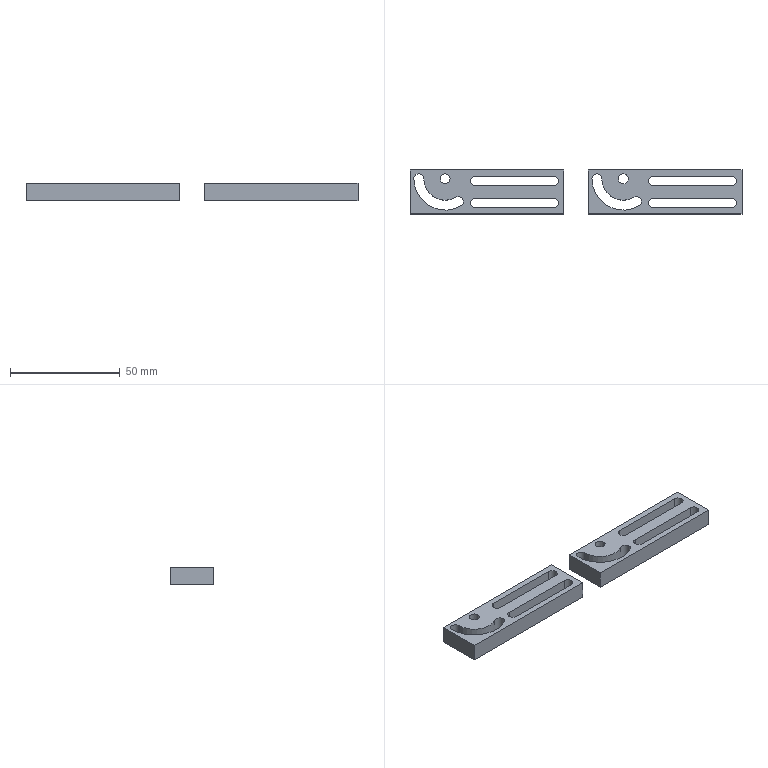Part | NX | 2 solids | 38 faces | box 151 x 20 x 8 mm | volume 14461 mm3 | plane 20 | cylinder 18 | commonest cylinder face diameters 4.5 x14 19.5 x2 28.5 x2
STEP:
#1=CARTESIAN_POINT('',(23.125,3.659,0.));
#2=VERTEX_POINT('',#1);
#3=CARTESIAN_POINT('',(1.75,16.,0.));
#4=VERTEX_POINT('',#3);
#5=CARTESIAN_POINT('',(16.,16.,0.));
#6=DIRECTION('',(0.,0.,-1.));
#7=DIRECTION('',(-1.,0.,0.));
#8=AXIS2_PLACEMENT_3D('',#5,#6,#7);
#9=CIRCLE('',#8,14.25);
#10=EDGE_CURVE('',#2,#4,#9,.T.);
#11=ORIENTED_EDGE('',*,*,#10,.T.);
#12=CARTESIAN_POINT('',(1.75,16.,8.));
#13=VERTEX_POINT('',#12);
#14=CARTESIAN_POINT('',(1.75,16.,8.));
#15=DIRECTION('',(0.,0.,-1.));
#16=VECTOR('',#15,1000.);
#17=LINE('',#14,#16);
#18=EDGE_CURVE('',#13,#4,#17,.T.);
#19=ORIENTED_EDGE('',*,*,#18,.F.);
#20=CARTESIAN_POINT('',(23.125,3.659,8.));
#21=VERTEX_POINT('',#20);
#22=CARTESIAN_POINT('',(16.,16.,8.));
#23=DIRECTION('',(0.,0.,-1.));
#24=DIRECTION('',(-1.,0.,0.));
#25=AXIS2_PLACEMENT_3D('',#22,#23,#24);
#26=CIRCLE('',#25,14.25);
#27=EDGE_CURVE('',#21,#13,#26,.T.);
#28=ORIENTED_EDGE('',*,*,#27,.F.);
#29=CARTESIAN_POINT('',(23.125,3.659,8.));
#30=DIRECTION('',(0.,0.,-1.));
#31=VECTOR('',#30,1000.);
#32=LINE('',#29,#31);
#33=EDGE_CURVE('',#21,#2,#32,.T.);
#34=ORIENTED_EDGE('',*,*,#33,.T.);
#35=EDGE_LOOP('',(#11,#19,#28,#34));
#36=FACE_BOUND('',#35,.T.);
#37=CARTESIAN_POINT('',(16.,16.,8.));
#38=DIRECTION('',(0.,0.,-1.));
#39=DIRECTION('',(-1.,0.,0.));
#40=AXIS2_PLACEMENT_3D('',#37,#38,#39);
#41=CYLINDRICAL_SURFACE('',#40,14.25);
#42=ADVANCED_FACE('',(#36),#41,.F.);
#43=CARTESIAN_POINT('',(6.25,16.,0.));
#44=VERTEX_POINT('',#43);
#45=CARTESIAN_POINT('',(4.,16.,0.));
#46=DIRECTION('',(0.,0.,-1.));
#47=DIRECTION('',(-1.,0.,0.));
#48=AXIS2_PLACEMENT_3D('',#45,#46,#47);
#49=CIRCLE('',#48,2.25);
#50=EDGE_CURVE('',#4,#44,#49,.T.);
#51=ORIENTED_EDGE('',*,*,#50,.T.);
#52=CARTESIAN_POINT('',(6.25,16.,8.));
#53=VERTEX_POINT('',#52);
#54=CARTESIAN_POINT('',(6.25,16.,8.));
#55=DIRECTION('',(0.,0.,-1.));
#56=VECTOR('',#55,1000.);
#57=LINE('',#54,#56);
#58=EDGE_CURVE('',#53,#44,#57,.T.);
#59=ORIENTED_EDGE('',*,*,#58,.F.);
#60=CARTESIAN_POINT('',(4.,16.,8.));
#61=DIRECTION('',(0.,0.,-1.));
#62=DIRECTION('',(-1.,0.,0.));
#63=AXIS2_PLACEMENT_3D('',#60,#61,#62);
#64=CIRCLE('',#63,2.25);
#65=EDGE_CURVE('',#13,#53,#64,.T.);
#66=ORIENTED_EDGE('',*,*,#65,.F.);
#67=ORIENTED_EDGE('',*,*,#18,.T.);
#68=EDGE_LOOP('',(#51,#59,#66,#67));
#69=FACE_BOUND('',#68,.T.);
#70=CARTESIAN_POINT('',(4.,16.,8.));
#71=DIRECTION('',(0.,0.,-1.));
#72=DIRECTION('',(-1.,0.,0.));
#73=AXIS2_PLACEMENT_3D('',#70,#71,#72);
#74=CYLINDRICAL_SURFACE('',#73,2.25);
#75=ADVANCED_FACE('',(#69),#74,.F.);
#76=CARTESIAN_POINT('',(20.875,7.556,0.));
#77=VERTEX_POINT('',#76);
#78=CARTESIAN_POINT('',(16.,16.,0.));
#79=DIRECTION('',(0.,0.,1.));
#80=DIRECTION('',(-1.,0.,0.));
#81=AXIS2_PLACEMENT_3D('',#78,#79,#80);
#82=CIRCLE('',#81,9.75);
#83=EDGE_CURVE('',#44,#77,#82,.T.);
#84=ORIENTED_EDGE('',*,*,#83,.T.);
#85=CARTESIAN_POINT('',(20.875,7.556,8.));
#86=VERTEX_POINT('',#85);
#87=CARTESIAN_POINT('',(20.875,7.556,8.));
#88=DIRECTION('',(0.,0.,-1.));
#89=VECTOR('',#88,1000.);
#90=LINE('',#87,#89);
#91=EDGE_CURVE('',#86,#77,#90,.T.);
#92=ORIENTED_EDGE('',*,*,#91,.F.);
#93=CARTESIAN_POINT('',(16.,16.,8.));
#94=DIRECTION('',(0.,0.,1.));
#95=DIRECTION('',(-1.,0.,0.));
#96=AXIS2_PLACEMENT_3D('',#93,#94,#95);
#97=CIRCLE('',#96,9.75);
#98=EDGE_CURVE('',#53,#86,#97,.T.);
#99=ORIENTED_EDGE('',*,*,#98,.F.);
#100=ORIENTED_EDGE('',*,*,#58,.T.);
#101=EDGE_LOOP('',(#84,#92,#99,#100));
#102=FACE_BOUND('',#101,.T.);
#103=CARTESIAN_POINT('',(16.,16.,8.));
#104=DIRECTION('',(0.,0.,-1.));
#105=DIRECTION('',(-1.,0.,0.));
#106=AXIS2_PLACEMENT_3D('',#103,#104,#105);
#107=CYLINDRICAL_SURFACE('',#106,9.75);
#108=ADVANCED_FACE('',(#102),#107,.T.);
#109=CARTESIAN_POINT('',(22.,5.608,0.));
#110=DIRECTION('',(0.,0.,-1.));
#111=DIRECTION('',(-1.,0.,0.));
#112=AXIS2_PLACEMENT_3D('',#109,#110,#111);
#113=CIRCLE('',#112,2.25);
#114=EDGE_CURVE('',#77,#2,#113,.T.);
#115=ORIENTED_EDGE('',*,*,#114,.T.);
#116=ORIENTED_EDGE('',*,*,#33,.F.);
#117=CARTESIAN_POINT('',(22.,5.608,8.));
#118=DIRECTION('',(0.,0.,-1.));
#119=DIRECTION('',(-1.,0.,0.));
#120=AXIS2_PLACEMENT_3D('',#117,#118,#119);
#121=CIRCLE('',#120,2.25);
#122=EDGE_CURVE('',#86,#21,#121,.T.);
#123=ORIENTED_EDGE('',*,*,#122,.F.);
#124=ORIENTED_EDGE('',*,*,#91,.T.);
#125=EDGE_LOOP('',(#115,#116,#123,#124));
#126=FACE_BOUND('',#125,.T.);
#127=CARTESIAN_POINT('',(22.,5.608,8.));
#128=DIRECTION('',(0.,0.,-1.));
#129=DIRECTION('',(-1.,0.,0.));
#130=AXIS2_PLACEMENT_3D('',#127,#128,#129);
#131=CYLINDRICAL_SURFACE('',#130,2.25);
#132=ADVANCED_FACE('',(#126),#131,.F.);
#133=CARTESIAN_POINT('',(65.25,12.75,8.));
#134=VERTEX_POINT('',#133);
#135=CARTESIAN_POINT('',(65.25,12.75,0.));
#136=VERTEX_POINT('',#135);
#137=CARTESIAN_POINT('',(65.25,12.75,8.));
#138=DIRECTION('',(0.,0.,-1.));
#139=VECTOR('',#138,1000.);
#140=LINE('',#137,#139);
#141=EDGE_CURVE('',#134,#136,#140,.T.);
#142=ORIENTED_EDGE('',*,*,#141,.T.);
#143=CARTESIAN_POINT('',(29.75,12.75,0.));
#144=VERTEX_POINT('',#143);
#145=CARTESIAN_POINT('',(29.75,12.75,0.));
#146=DIRECTION('',(1.,0.,0.));
#147=VECTOR('',#146,1000.);
#148=LINE('',#145,#147);
#149=EDGE_CURVE('',#144,#136,#148,.T.);
#150=ORIENTED_EDGE('',*,*,#149,.F.);
#151=CARTESIAN_POINT('',(29.75,12.75,8.));
#152=VERTEX_POINT('',#151);
#153=CARTESIAN_POINT('',(29.75,12.75,8.));
#154=DIRECTION('',(0.,0.,1.));
#155=VECTOR('',#154,1000.);
#156=LINE('',#153,#155);
#157=EDGE_CURVE('',#144,#152,#156,.T.);
#158=ORIENTED_EDGE('',*,*,#157,.T.);
#159=CARTESIAN_POINT('',(29.75,12.75,8.));
#160=DIRECTION('',(1.,0.,0.));
#161=VECTOR('',#160,1000.);
#162=LINE('',#159,#161);
#163=EDGE_CURVE('',#152,#134,#162,.T.);
#164=ORIENTED_EDGE('',*,*,#163,.T.);
#165=EDGE_LOOP('',(#142,#150,#158,#164));
#166=FACE_BOUND('',#165,.T.);
#167=CARTESIAN_POINT('',(29.75,12.75,8.));
#168=DIRECTION('',(0.,-1.,0.));
#169=DIRECTION('',(1.,0.,0.));
#170=AXIS2_PLACEMENT_3D('',#167,#168,#169);
#171=PLANE('',#170);
#172=ADVANCED_FACE('',(#166),#171,.F.);
#173=CARTESIAN_POINT('',(65.25,17.25,0.));
#174=VERTEX_POINT('',#173);
#175=CARTESIAN_POINT('',(65.25,17.25,8.));
#176=VERTEX_POINT('',#175);
#177=CARTESIAN_POINT('',(65.25,17.25,8.));
#178=DIRECTION('',(0.,0.,1.));
#179=VECTOR('',#178,1000.);
#180=LINE('',#177,#179);
#181=EDGE_CURVE('',#174,#176,#180,.T.);
#182=ORIENTED_EDGE('',*,*,#181,.T.);
#183=CARTESIAN_POINT('',(29.75,17.25,8.));
#184=VERTEX_POINT('',#183);
#185=CARTESIAN_POINT('',(29.75,17.25,8.));
#186=DIRECTION('',(1.,0.,0.));
#187=VECTOR('',#186,1000.);
#188=LINE('',#185,#187);
#189=EDGE_CURVE('',#184,#176,#188,.T.);
#190=ORIENTED_EDGE('',*,*,#189,.F.);
#191=CARTESIAN_POINT('',(29.75,17.25,0.));
#192=VERTEX_POINT('',#191);
#193=CARTESIAN_POINT('',(29.75,17.25,8.));
#194=DIRECTION('',(0.,0.,-1.));
#195=VECTOR('',#194,1000.);
#196=LINE('',#193,#195);
#197=EDGE_CURVE('',#184,#192,#196,.T.);
#198=ORIENTED_EDGE('',*,*,#197,.T.);
#199=CARTESIAN_POINT('',(29.75,17.25,0.));
#200=DIRECTION('',(1.,0.,0.));
#201=VECTOR('',#200,1000.);
#202=LINE('',#199,#201);
#203=EDGE_CURVE('',#192,#174,#202,.T.);
#204=ORIENTED_EDGE('',*,*,#203,.T.);
#205=EDGE_LOOP('',(#182,#190,#198,#204));
#206=FACE_BOUND('',#205,.T.);
#207=CARTESIAN_POINT('',(29.75,17.25,8.));
#208=DIRECTION('',(0.,1.,0.));
#209=DIRECTION('',(-1.,0.,0.));
#210=AXIS2_PLACEMENT_3D('',#207,#208,#209);
#211=PLANE('',#210);
#212=ADVANCED_FACE('',(#206),#211,.F.);
#213=CARTESIAN_POINT('',(29.75,15.,8.));
#214=DIRECTION('',(0.,0.,1.));
#215=DIRECTION('',(1.,0.,0.));
#216=AXIS2_PLACEMENT_3D('',#213,#214,#215);
#217=CIRCLE('',#216,2.25);
#218=EDGE_CURVE('',#184,#152,#217,.T.);
#219=ORIENTED_EDGE('',*,*,#218,.T.);
#220=ORIENTED_EDGE('',*,*,#157,.F.);
#221=CARTESIAN_POINT('',(29.75,15.,0.));
#222=DIRECTION('',(0.,0.,1.));
#223=DIRECTION('',(1.,0.,0.));
#224=AXIS2_PLACEMENT_3D('',#221,#222,#223);
#225=CIRCLE('',#224,2.25);
#226=EDGE_CURVE('',#192,#144,#225,.T.);
#227=ORIENTED_EDGE('',*,*,#226,.F.);
#228=ORIENTED_EDGE('',*,*,#197,.F.);
#229=EDGE_LOOP('',(#219,#220,#227,#228));
#230=FACE_BOUND('',#229,.T.);
#231=CARTESIAN_POINT('',(29.75,15.,8.));
#232=DIRECTION('',(0.,0.,1.));
#233=DIRECTION('',(1.,0.,0.));
#234=AXIS2_PLACEMENT_3D('',#231,#232,#233);
#235=CYLINDRICAL_SURFACE('',#234,2.25);
#236=ADVANCED_FACE('',(#230),#235,.F.);
#237=CARTESIAN_POINT('',(65.25,2.75,8.));
#238=VERTEX_POINT('',#237);
#239=CARTESIAN_POINT('',(65.25,2.75,0.));
#240=VERTEX_POINT('',#239);
#241=CARTESIAN_POINT('',(65.25,2.75,8.));
#242=DIRECTION('',(0.,0.,-1.));
#243=VECTOR('',#242,1000.);
#244=LINE('',#241,#243);
#245=EDGE_CURVE('',#238,#240,#244,.T.);
#246=ORIENTED_EDGE('',*,*,#245,.T.);
#247=CARTESIAN_POINT('',(29.75,2.75,0.));
#248=VERTEX_POINT('',#247);
#249=CARTESIAN_POINT('',(29.75,2.75,0.));
#250=DIRECTION('',(1.,0.,0.));
#251=VECTOR('',#250,1000.);
#252=LINE('',#249,#251);
#253=EDGE_CURVE('',#248,#240,#252,.T.);
#254=ORIENTED_EDGE('',*,*,#253,.F.);
#255=CARTESIAN_POINT('',(29.75,2.75,8.));
#256=VERTEX_POINT('',#255);
#257=CARTESIAN_POINT('',(29.75,2.75,8.));
#258=DIRECTION('',(0.,0.,1.));
#259=VECTOR('',#258,1000.);
#260=LINE('',#257,#259);
#261=EDGE_CURVE('',#248,#256,#260,.T.);
#262=ORIENTED_EDGE('',*,*,#261,.T.);
#263=CARTESIAN_POINT('',(29.75,2.75,8.));
#264=DIRECTION('',(1.,0.,0.));
#265=VECTOR('',#264,1000.);
#266=LINE('',#263,#265);
#267=EDGE_CURVE('',#256,#238,#266,.T.);
#268=ORIENTED_EDGE('',*,*,#267,.T.);
#269=EDGE_LOOP('',(#246,#254,#262,#268));
#270=FACE_BOUND('',#269,.T.);
#271=CARTESIAN_POINT('',(29.75,2.75,8.));
#272=DIRECTION('',(0.,-1.,0.));
#273=DIRECTION('',(1.,0.,0.));
#274=AXIS2_PLACEMENT_3D('',#271,#272,#273);
#275=PLANE('',#274);
#276=ADVANCED_FACE('',(#270),#275,.F.);
#277=CARTESIAN_POINT('',(65.25,7.25,0.));
#278=VERTEX_POINT('',#277);
#279=CARTESIAN_POINT('',(65.25,7.25,8.));
#280=VERTEX_POINT('',#279);
#281=CARTESIAN_POINT('',(65.25,7.25,8.));
#282=DIRECTION('',(0.,0.,1.));
#283=VECTOR('',#282,1000.);
#284=LINE('',#281,#283);
#285=EDGE_CURVE('',#278,#280,#284,.T.);
#286=ORIENTED_EDGE('',*,*,#285,.T.);
#287=CARTESIAN_POINT('',(29.75,7.25,8.));
#288=VERTEX_POINT('',#287);
#289=CARTESIAN_POINT('',(29.75,7.25,8.));
#290=DIRECTION('',(1.,0.,0.));
#291=VECTOR('',#290,1000.);
#292=LINE('',#289,#291);
#293=EDGE_CURVE('',#288,#280,#292,.T.);
#294=ORIENTED_EDGE('',*,*,#293,.F.);
#295=CARTESIAN_POINT('',(29.75,7.25,0.));
#296=VERTEX_POINT('',#295);
#297=CARTESIAN_POINT('',(29.75,7.25,8.));
#298=DIRECTION('',(0.,0.,-1.));
#299=VECTOR('',#298,1000.);
#300=LINE('',#297,#299);
#301=EDGE_CURVE('',#288,#296,#300,.T.);
#302=ORIENTED_EDGE('',*,*,#301,.T.);
#303=CARTESIAN_POINT('',(29.75,7.25,0.));
#304=DIRECTION('',(1.,0.,0.));
#305=VECTOR('',#304,1000.);
#306=LINE('',#303,#305);
#307=EDGE_CURVE('',#296,#278,#306,.T.);
#308=ORIENTED_EDGE('',*,*,#307,.T.);
#309=EDGE_LOOP('',(#286,#294,#302,#308));
#310=FACE_BOUND('',#309,.T.);
#311=CARTESIAN_POINT('',(29.75,7.25,8.));
#312=DIRECTION('',(0.,1.,0.));
#313=DIRECTION('',(-1.,0.,0.));
#314=AXIS2_PLACEMENT_3D('',#311,#312,#313);
#315=PLANE('',#314);
#316=ADVANCED_FACE('',(#310),#315,.F.);
#317=CARTESIAN_POINT('',(29.75,5.,8.));
#318=DIRECTION('',(0.,0.,1.));
#319=DIRECTION('',(1.,0.,0.));
#320=AXIS2_PLACEMENT_3D('',#317,#318,#319);
#321=CIRCLE('',#320,2.25);
#322=EDGE_CURVE('',#288,#256,#321,.T.);
#323=ORIENTED_EDGE('',*,*,#322,.T.);
#324=ORIENTED_EDGE('',*,*,#261,.F.);
#325=CARTESIAN_POINT('',(29.75,5.,0.));
#326=DIRECTION('',(0.,0.,1.));
#327=DIRECTION('',(1.,0.,0.));
#328=AXIS2_PLACEMENT_3D('',#325,#326,#327);
#329=CIRCLE('',#328,2.25);
#330=EDGE_CURVE('',#296,#248,#329,.T.);
#331=ORIENTED_EDGE('',*,*,#330,.F.);
#332=ORIENTED_EDGE('',*,*,#301,.F.);
#333=EDGE_LOOP('',(#323,#324,#331,#332));
#334=FACE_BOUND('',#333,.T.);
#335=CARTESIAN_POINT('',(29.75,5.,8.));
#336=DIRECTION('',(0.,0.,1.));
#337=DIRECTION('',(1.,0.,0.));
#338=AXIS2_PLACEMENT_3D('',#335,#336,#337);
#339=CYLINDRICAL_SURFACE('',#338,2.25);
#340=ADVANCED_FACE('',(#334),#339,.F.);
#341=CARTESIAN_POINT('',(0.,20.,0.));
#342=VERTEX_POINT('',#341);
#343=CARTESIAN_POINT('',(0.,0.,0.));
#344=VERTEX_POINT('',#343);
#345=CARTESIAN_POINT('',(0.,20.,0.));
#346=DIRECTION('',(0.,-1.,0.));
#347=VECTOR('',#346,1000.);
#348=LINE('',#345,#347);
#349=EDGE_CURVE('',#342,#344,#348,.T.);
#350=ORIENTED_EDGE('',*,*,#349,.F.);
#351=CARTESIAN_POINT('',(70.,20.,0.));
#352=VERTEX_POINT('',#351);
#353=CARTESIAN_POINT('',(70.,20.,0.));
#354=DIRECTION('',(-1.,0.,0.));
#355=VECTOR('',#354,1000.);
#356=LINE('',#353,#355);
#357=EDGE_CURVE('',#352,#342,#356,.T.);
#358=ORIENTED_EDGE('',*,*,#357,.F.);
#359=CARTESIAN_POINT('',(70.,0.,0.));
#360=VERTEX_POINT('',#359);
#361=CARTESIAN_POINT('',(70.,0.,0.));
#362=DIRECTION('',(0.,1.,0.));
#363=VECTOR('',#362,1000.);
#364=LINE('',#361,#363);
#365=EDGE_CURVE('',#360,#352,#364,.T.);
#366=ORIENTED_EDGE('',*,*,#365,.F.);
#367=CARTESIAN_POINT('',(0.,0.,0.));
#368=DIRECTION('',(1.,0.,0.));
#369=VECTOR('',#368,1000.);
#370=LINE('',#367,#369);
#371=EDGE_CURVE('',#344,#360,#370,.T.);
#372=ORIENTED_EDGE('',*,*,#371,.F.);
#373=EDGE_LOOP('',(#350,#358,#366,#372));
#374=FACE_BOUND('',#373,.T.);
#375=ORIENTED_EDGE('',*,*,#253,.T.);
#376=CARTESIAN_POINT('',(65.25,5.,0.));
#377=DIRECTION('',(0.,0.,1.));
#378=DIRECTION('',(1.,0.,0.));
#379=AXIS2_PLACEMENT_3D('',#376,#377,#378);
#380=CIRCLE('',#379,2.25);
#381=EDGE_CURVE('',#240,#278,#380,.T.);
#382=ORIENTED_EDGE('',*,*,#381,.T.);
#383=ORIENTED_EDGE('',*,*,#307,.F.);
#384=ORIENTED_EDGE('',*,*,#330,.T.);
#385=EDGE_LOOP('',(#375,#382,#383,#384));
#386=FACE_BOUND('',#385,.T.);
#387=ORIENTED_EDGE('',*,*,#149,.T.);
#388=CARTESIAN_POINT('',(65.25,15.,0.));
#389=DIRECTION('',(0.,0.,1.));
#390=DIRECTION('',(1.,0.,0.));
#391=AXIS2_PLACEMENT_3D('',#388,#389,#390);
#392=CIRCLE('',#391,2.25);
#393=EDGE_CURVE('',#136,#174,#392,.T.);
#394=ORIENTED_EDGE('',*,*,#393,.T.);
#395=ORIENTED_EDGE('',*,*,#203,.F.);
#396=ORIENTED_EDGE('',*,*,#226,.T.);
#397=EDGE_LOOP('',(#387,#394,#395,#396));
#398=FACE_BOUND('',#397,.T.);
#399=CARTESIAN_POINT('',(13.75,16.,0.));
#400=VERTEX_POINT('',#399);
#401=CARTESIAN_POINT('',(16.,16.,0.));
#402=DIRECTION('',(0.,0.,-1.));
#403=DIRECTION('',(-1.,0.,0.));
#404=AXIS2_PLACEMENT_3D('',#401,#402,#403);
#405=CIRCLE('',#404,2.25);
#406=EDGE_CURVE('',#400,#400,#405,.T.);
#407=ORIENTED_EDGE('',*,*,#406,.F.);
#408=EDGE_LOOP('',(#407));
#409=FACE_BOUND('',#408,.T.);
#410=ORIENTED_EDGE('',*,*,#10,.F.);
#411=ORIENTED_EDGE('',*,*,#114,.F.);
#412=ORIENTED_EDGE('',*,*,#83,.F.);
#413=ORIENTED_EDGE('',*,*,#50,.F.);
#414=EDGE_LOOP('',(#410,#411,#412,#413));
#415=FACE_BOUND('',#414,.T.);
#416=CARTESIAN_POINT('',(0.,0.,0.));
#417=DIRECTION('',(0.,0.,1.));
#418=DIRECTION('',(1.,0.,0.));
#419=AXIS2_PLACEMENT_3D('',#416,#417,#418);
#420=PLANE('',#419);
#421=ADVANCED_FACE('',(#374,#386,#398,#409,#415),#420,.F.);
#422=CARTESIAN_POINT('',(0.,20.,8.));
#423=VERTEX_POINT('',#422);
#424=CARTESIAN_POINT('',(0.,0.,8.));
#425=VERTEX_POINT('',#424);
#426=CARTESIAN_POINT('',(0.,20.,8.));
#427=DIRECTION('',(0.,-1.,0.));
#428=VECTOR('',#427,1000.);
#429=LINE('',#426,#428);
#430=EDGE_CURVE('',#423,#425,#429,.T.);
#431=ORIENTED_EDGE('',*,*,#430,.T.);
#432=CARTESIAN_POINT('',(70.,0.,8.));
#433=VERTEX_POINT('',#432);
#434=CARTESIAN_POINT('',(0.,0.,8.));
#435=DIRECTION('',(1.,0.,0.));
#436=VECTOR('',#435,1000.);
#437=LINE('',#434,#436);
#438=EDGE_CURVE('',#425,#433,#437,.T.);
#439=ORIENTED_EDGE('',*,*,#438,.T.);
#440=CARTESIAN_POINT('',(70.,20.,8.));
#441=VERTEX_POINT('',#440);
#442=CARTESIAN_POINT('',(70.,0.,8.));
#443=DIRECTION('',(0.,1.,0.));
#444=VECTOR('',#443,1000.);
#445=LINE('',#442,#444);
#446=EDGE_CURVE('',#433,#441,#445,.T.);
#447=ORIENTED_EDGE('',*,*,#446,.T.);
#448=CARTESIAN_POINT('',(70.,20.,8.));
#449=DIRECTION('',(-1.,0.,0.));
#450=VECTOR('',#449,1000.);
#451=LINE('',#448,#450);
#452=EDGE_CURVE('',#441,#423,#451,.T.);
#453=ORIENTED_EDGE('',*,*,#452,.T.);
#454=EDGE_LOOP('',(#431,#439,#447,#453));
#455=FACE_BOUND('',#454,.T.);
#456=ORIENTED_EDGE('',*,*,#322,.F.);
#457=ORIENTED_EDGE('',*,*,#293,.T.);
#458=CARTESIAN_POINT('',(65.25,5.,8.));
#459=DIRECTION('',(0.,0.,1.));
#460=DIRECTION('',(1.,0.,0.));
#461=AXIS2_PLACEMENT_3D('',#458,#459,#460);
#462=CIRCLE('',#461,2.25);
#463=EDGE_CURVE('',#238,#280,#462,.T.);
#464=ORIENTED_EDGE('',*,*,#463,.F.);
#465=ORIENTED_EDGE('',*,*,#267,.F.);
#466=EDGE_LOOP('',(#456,#457,#464,#465));
#467=FACE_BOUND('',#466,.T.);
#468=ORIENTED_EDGE('',*,*,#163,.F.);
#469=ORIENTED_EDGE('',*,*,#218,.F.);
#470=ORIENTED_EDGE('',*,*,#189,.T.);
#471=CARTESIAN_POINT('',(65.25,15.,8.));
#472=DIRECTION('',(0.,0.,1.));
#473=DIRECTION('',(1.,0.,0.));
#474=AXIS2_PLACEMENT_3D('',#471,#472,#473);
#475=CIRCLE('',#474,2.25);
#476=EDGE_CURVE('',#134,#176,#475,.T.);
#477=ORIENTED_EDGE('',*,*,#476,.F.);
#478=EDGE_LOOP('',(#468,#469,#470,#477));
#479=FACE_BOUND('',#478,.T.);
#480=CARTESIAN_POINT('',(13.75,16.,8.));
#481=VERTEX_POINT('',#480);
#482=CARTESIAN_POINT('',(16.,16.,8.));
#483=DIRECTION('',(0.,0.,-1.));
#484=DIRECTION('',(-1.,0.,0.));
#485=AXIS2_PLACEMENT_3D('',#482,#483,#484);
#486=CIRCLE('',#485,2.25);
#487=EDGE_CURVE('',#481,#481,#486,.T.);
#488=ORIENTED_EDGE('',*,*,#487,.T.);
#489=EDGE_LOOP('',(#488));
#490=FACE_BOUND('',#489,.T.);
#491=ORIENTED_EDGE('',*,*,#122,.T.);
#492=ORIENTED_EDGE('',*,*,#27,.T.);
#493=ORIENTED_EDGE('',*,*,#65,.T.);
#494=ORIENTED_EDGE('',*,*,#98,.T.);
#495=EDGE_LOOP('',(#491,#492,#493,#494));
#496=FACE_BOUND('',#495,.T.);
#497=CARTESIAN_POINT('',(0.,0.,8.));
#498=DIRECTION('',(0.,0.,1.));
#499=DIRECTION('',(1.,0.,0.));
#500=AXIS2_PLACEMENT_3D('',#497,#498,#499);
#501=PLANE('',#500);
#502=ADVANCED_FACE('',(#455,#467,#479,#490,#496),#501,.T.);
#503=ORIENTED_EDGE('',*,*,#357,.T.);
#504=CARTESIAN_POINT('',(0.,20.,8.));
#505=DIRECTION('',(0.,0.,-1.));
#506=VECTOR('',#505,1000.);
#507=LINE('',#504,#506);
#508=EDGE_CURVE('',#423,#342,#507,.T.);
#509=ORIENTED_EDGE('',*,*,#508,.F.);
#510=ORIENTED_EDGE('',*,*,#452,.F.);
#511=CARTESIAN_POINT('',(70.,20.,8.));
#512=DIRECTION('',(0.,0.,-1.));
#513=VECTOR('',#512,1000.);
#514=LINE('',#511,#513);
#515=EDGE_CURVE('',#441,#352,#514,.T.);
#516=ORIENTED_EDGE('',*,*,#515,.T.);
#517=EDGE_LOOP('',(#503,#509,#510,#516));
#518=FACE_BOUND('',#517,.T.);
#519=CARTESIAN_POINT('',(70.,20.,8.));
#520=DIRECTION('',(0.,-1.,0.));
#521=DIRECTION('',(1.,0.,0.));
#522=AXIS2_PLACEMENT_3D('',#519,#520,#521);
#523=PLANE('',#522);
#524=ADVANCED_FACE('',(#518),#523,.F.);
#525=ORIENTED_EDGE('',*,*,#365,.T.);
#526=ORIENTED_EDGE('',*,*,#515,.F.);
#527=ORIENTED_EDGE('',*,*,#446,.F.);
#528=CARTESIAN_POINT('',(70.,0.,8.));
#529=DIRECTION('',(0.,0.,-1.));
#530=VECTOR('',#529,1000.);
#531=LINE('',#528,#530);
#532=EDGE_CURVE('',#433,#360,#531,.T.);
#533=ORIENTED_EDGE('',*,*,#532,.T.);
#534=EDGE_LOOP('',(#525,#526,#527,#533));
#535=FACE_BOUND('',#534,.T.);
#536=CARTESIAN_POINT('',(70.,0.,8.));
#537=DIRECTION('',(-1.,0.,0.));
#538=DIRECTION('',(0.,0.,1.));
#539=AXIS2_PLACEMENT_3D('',#536,#537,#538);
#540=PLANE('',#539);
#541=ADVANCED_FACE('',(#535),#540,.F.);
#542=ORIENTED_EDGE('',*,*,#371,.T.);
#543=ORIENTED_EDGE('',*,*,#532,.F.);
#544=ORIENTED_EDGE('',*,*,#438,.F.);
#545=CARTESIAN_POINT('',(0.,0.,8.));
#546=DIRECTION('',(0.,0.,-1.));
#547=VECTOR('',#546,1000.);
#548=LINE('',#545,#547);
#549=EDGE_CURVE('',#425,#344,#548,.T.);
#550=ORIENTED_EDGE('',*,*,#549,.T.);
#551=EDGE_LOOP('',(#542,#543,#544,#550));
#552=FACE_BOUND('',#551,.T.);
#553=CARTESIAN_POINT('',(0.,0.,8.));
#554=DIRECTION('',(0.,1.,0.));
#555=DIRECTION('',(0.,0.,1.));
#556=AXIS2_PLACEMENT_3D('',#553,#554,#555);
#557=PLANE('',#556);
#558=ADVANCED_FACE('',(#552),#557,.F.);
#559=ORIENTED_EDGE('',*,*,#349,.T.);
#560=ORIENTED_EDGE('',*,*,#549,.F.);
#561=ORIENTED_EDGE('',*,*,#430,.F.);
#562=ORIENTED_EDGE('',*,*,#508,.T.);
#563=EDGE_LOOP('',(#559,#560,#561,#562));
#564=FACE_BOUND('',#563,.T.);
#565=CARTESIAN_POINT('',(0.,20.,8.));
#566=DIRECTION('',(1.,0.,0.));
#567=DIRECTION('',(0.,0.,-1.));
#568=AXIS2_PLACEMENT_3D('',#565,#566,#567);
#569=PLANE('',#568);
#570=ADVANCED_FACE('',(#564),#569,.F.);
#571=ORIENTED_EDGE('',*,*,#381,.F.);
#572=ORIENTED_EDGE('',*,*,#245,.F.);
#573=ORIENTED_EDGE('',*,*,#463,.T.);
#574=ORIENTED_EDGE('',*,*,#285,.F.);
#575=EDGE_LOOP('',(#571,#572,#573,#574));
#576=FACE_BOUND('',#575,.T.);
#577=CARTESIAN_POINT('',(65.25,5.,8.));
#578=DIRECTION('',(0.,0.,1.));
#579=DIRECTION('',(1.,0.,0.));
#580=AXIS2_PLACEMENT_3D('',#577,#578,#579);
#581=CYLINDRICAL_SURFACE('',#580,2.25);
#582=ADVANCED_FACE('',(#576),#581,.F.);
#583=ORIENTED_EDGE('',*,*,#393,.F.);
#584=ORIENTED_EDGE('',*,*,#141,.F.);
#585=ORIENTED_EDGE('',*,*,#476,.T.);
#586=ORIENTED_EDGE('',*,*,#181,.F.);
#587=EDGE_LOOP('',(#583,#584,#585,#586));
#588=FACE_BOUND('',#587,.T.);
#589=CARTESIAN_POINT('',(65.25,15.,8.));
#590=DIRECTION('',(0.,0.,1.));
#591=DIRECTION('',(1.,0.,0.));
#592=AXIS2_PLACEMENT_3D('',#589,#590,#591);
#593=CYLINDRICAL_SURFACE('',#592,2.25);
#594=ADVANCED_FACE('',(#588),#593,.F.);
#595=ORIENTED_EDGE('',*,*,#406,.T.);
#596=EDGE_LOOP('',(#595));
#597=FACE_BOUND('',#596,.T.);
#598=ORIENTED_EDGE('',*,*,#487,.F.);
#599=EDGE_LOOP('',(#598));
#600=FACE_BOUND('',#599,.T.);
#601=CARTESIAN_POINT('',(16.,16.,0.));
#602=DIRECTION('',(0.,0.,-1.));
#603=DIRECTION('',(-1.,0.,0.));
#604=AXIS2_PLACEMENT_3D('',#601,#602,#603);
#605=CYLINDRICAL_SURFACE('',#604,2.25);
#606=ADVANCED_FACE('',(#597,#600),#605,.F.);
#607=CLOSED_SHELL('',(#42,#75,#108,#132,#172,#212,#236,#276,#316,#340,#421,#502,#524,#541,#558,#570,#582,#594,#606));
#608=MANIFOLD_SOLID_BREP('',#607);
#609=CARTESIAN_POINT('',(104.125,3.659,0.));
#610=VERTEX_POINT('',#609);
#611=CARTESIAN_POINT('',(82.75,16.,0.));
#612=VERTEX_POINT('',#611);
#613=CARTESIAN_POINT('',(97.,16.,0.));
#614=DIRECTION('',(0.,0.,-1.));
#615=DIRECTION('',(-1.,0.,0.));
#616=AXIS2_PLACEMENT_3D('',#613,#614,#615);
#617=CIRCLE('',#616,14.25);
#618=EDGE_CURVE('',#610,#612,#617,.T.);
#619=ORIENTED_EDGE('',*,*,#618,.T.);
#620=CARTESIAN_POINT('',(82.75,16.,8.));
#621=VERTEX_POINT('',#620);
#622=CARTESIAN_POINT('',(82.75,16.,8.));
#623=DIRECTION('',(0.,0.,-1.));
#624=VECTOR('',#623,1000.);
#625=LINE('',#622,#624);
#626=EDGE_CURVE('',#621,#612,#625,.T.);
#627=ORIENTED_EDGE('',*,*,#626,.F.);
#628=CARTESIAN_POINT('',(104.125,3.659,8.));
#629=VERTEX_POINT('',#628);
#630=CARTESIAN_POINT('',(97.,16.,8.));
#631=DIRECTION('',(0.,0.,-1.));
#632=DIRECTION('',(-1.,0.,0.));
#633=AXIS2_PLACEMENT_3D('',#630,#631,#632);
#634=CIRCLE('',#633,14.25);
#635=EDGE_CURVE('',#629,#621,#634,.T.);
#636=ORIENTED_EDGE('',*,*,#635,.F.);
#637=CARTESIAN_POINT('',(104.125,3.659,8.));
#638=DIRECTION('',(0.,0.,-1.));
#639=VECTOR('',#638,1000.);
#640=LINE('',#637,#639);
#641=EDGE_CURVE('',#629,#610,#640,.T.);
#642=ORIENTED_EDGE('',*,*,#641,.T.);
#643=EDGE_LOOP('',(#619,#627,#636,#642));
#644=FACE_BOUND('',#643,.T.);
#645=CARTESIAN_POINT('',(97.,16.,8.));
#646=DIRECTION('',(0.,0.,-1.));
#647=DIRECTION('',(-1.,0.,0.));
#648=AXIS2_PLACEMENT_3D('',#645,#646,#647);
#649=CYLINDRICAL_SURFACE('',#648,14.25);
#650=ADVANCED_FACE('',(#644),#649,.F.);
#651=CARTESIAN_POINT('',(87.25,16.,0.));
#652=VERTEX_POINT('',#651);
#653=CARTESIAN_POINT('',(85.,16.,0.));
#654=DIRECTION('',(0.,0.,-1.));
#655=DIRECTION('',(-1.,0.,0.));
#656=AXIS2_PLACEMENT_3D('',#653,#654,#655);
#657=CIRCLE('',#656,2.25);
#658=EDGE_CURVE('',#612,#652,#657,.T.);
#659=ORIENTED_EDGE('',*,*,#658,.T.);
#660=CARTESIAN_POINT('',(87.25,16.,8.));
#661=VERTEX_POINT('',#660);
#662=CARTESIAN_POINT('',(87.25,16.,8.));
#663=DIRECTION('',(0.,0.,-1.));
#664=VECTOR('',#663,1000.);
#665=LINE('',#662,#664);
#666=EDGE_CURVE('',#661,#652,#665,.T.);
#667=ORIENTED_EDGE('',*,*,#666,.F.);
#668=CARTESIAN_POINT('',(85.,16.,8.));
#669=DIRECTION('',(0.,0.,-1.));
#670=DIRECTION('',(-1.,0.,0.));
#671=AXIS2_PLACEMENT_3D('',#668,#669,#670);
#672=CIRCLE('',#671,2.25);
#673=EDGE_CURVE('',#621,#661,#672,.T.);
#674=ORIENTED_EDGE('',*,*,#673,.F.);
#675=ORIENTED_EDGE('',*,*,#626,.T.);
#676=EDGE_LOOP('',(#659,#667,#674,#675));
#677=FACE_BOUND('',#676,.T.);
#678=CARTESIAN_POINT('',(85.,16.,8.));
#679=DIRECTION('',(0.,0.,-1.));
#680=DIRECTION('',(-1.,0.,0.));
#681=AXIS2_PLACEMENT_3D('',#678,#679,#680);
#682=CYLINDRICAL_SURFACE('',#681,2.25);
#683=ADVANCED_FACE('',(#677),#682,.F.);
#684=CARTESIAN_POINT('',(101.875,7.556,0.));
#685=VERTEX_POINT('',#684);
#686=CARTESIAN_POINT('',(97.,16.,0.));
#687=DIRECTION('',(0.,0.,1.));
#688=DIRECTION('',(-1.,0.,0.));
#689=AXIS2_PLACEMENT_3D('',#686,#687,#688);
#690=CIRCLE('',#689,9.75);
#691=EDGE_CURVE('',#652,#685,#690,.T.);
#692=ORIENTED_EDGE('',*,*,#691,.T.);
#693=CARTESIAN_POINT('',(101.875,7.556,8.));
#694=VERTEX_POINT('',#693);
#695=CARTESIAN_POINT('',(101.875,7.556,8.));
#696=DIRECTION('',(0.,0.,-1.));
#697=VECTOR('',#696,1000.);
#698=LINE('',#695,#697);
#699=EDGE_CURVE('',#694,#685,#698,.T.);
#700=ORIENTED_EDGE('',*,*,#699,.F.);
#701=CARTESIAN_POINT('',(97.,16.,8.));
#702=DIRECTION('',(0.,0.,1.));
#703=DIRECTION('',(-1.,0.,0.));
#704=AXIS2_PLACEMENT_3D('',#701,#702,#703);
#705=CIRCLE('',#704,9.75);
#706=EDGE_CURVE('',#661,#694,#705,.T.);
#707=ORIENTED_EDGE('',*,*,#706,.F.);
#708=ORIENTED_EDGE('',*,*,#666,.T.);
#709=EDGE_LOOP('',(#692,#700,#707,#708));
#710=FACE_BOUND('',#709,.T.);
#711=CARTESIAN_POINT('',(97.,16.,8.));
#712=DIRECTION('',(0.,0.,-1.));
#713=DIRECTION('',(-1.,0.,0.));
#714=AXIS2_PLACEMENT_3D('',#711,#712,#713);
#715=CYLINDRICAL_SURFACE('',#714,9.75);
#716=ADVANCED_FACE('',(#710),#715,.T.);
#717=CARTESIAN_POINT('',(103.,5.608,0.));
#718=DIRECTION('',(0.,0.,-1.));
#719=DIRECTION('',(-1.,0.,0.));
#720=AXIS2_PLACEMENT_3D('',#717,#718,#719);
#721=CIRCLE('',#720,2.25);
#722=EDGE_CURVE('',#685,#610,#721,.T.);
#723=ORIENTED_EDGE('',*,*,#722,.T.);
#724=ORIENTED_EDGE('',*,*,#641,.F.);
#725=CARTESIAN_POINT('',(103.,5.608,8.));
#726=DIRECTION('',(0.,0.,-1.));
#727=DIRECTION('',(-1.,0.,0.));
#728=AXIS2_PLACEMENT_3D('',#725,#726,#727);
#729=CIRCLE('',#728,2.25);
#730=EDGE_CURVE('',#694,#629,#729,.T.);
#731=ORIENTED_EDGE('',*,*,#730,.F.);
#732=ORIENTED_EDGE('',*,*,#699,.T.);
#733=EDGE_LOOP('',(#723,#724,#731,#732));
#734=FACE_BOUND('',#733,.T.);
#735=CARTESIAN_POINT('',(103.,5.608,8.));
#736=DIRECTION('',(0.,0.,-1.));
#737=DIRECTION('',(-1.,0.,0.));
#738=AXIS2_PLACEMENT_3D('',#735,#736,#737);
#739=CYLINDRICAL_SURFACE('',#738,2.25);
#740=ADVANCED_FACE('',(#734),#739,.F.);
#741=CARTESIAN_POINT('',(146.25,12.75,8.));
#742=VERTEX_POINT('',#741);
#743=CARTESIAN_POINT('',(146.25,12.75,0.));
#744=VERTEX_POINT('',#743);
#745=CARTESIAN_POINT('',(146.25,12.75,8.));
#746=DIRECTION('',(0.,0.,-1.));
#747=VECTOR('',#746,1000.);
#748=LINE('',#745,#747);
#749=EDGE_CURVE('',#742,#744,#748,.T.);
#750=ORIENTED_EDGE('',*,*,#749,.T.);
#751=CARTESIAN_POINT('',(110.75,12.75,0.));
#752=VERTEX_POINT('',#751);
#753=CARTESIAN_POINT('',(110.75,12.75,0.));
#754=DIRECTION('',(1.,0.,0.));
#755=VECTOR('',#754,1000.);
#756=LINE('',#753,#755);
#757=EDGE_CURVE('',#752,#744,#756,.T.);
#758=ORIENTED_EDGE('',*,*,#757,.F.);
#759=CARTESIAN_POINT('',(110.75,12.75,8.));
#760=VERTEX_POINT('',#759);
#761=CARTESIAN_POINT('',(110.75,12.75,8.));
#762=DIRECTION('',(0.,0.,1.));
#763=VECTOR('',#762,1000.);
#764=LINE('',#761,#763);
#765=EDGE_CURVE('',#752,#760,#764,.T.);
#766=ORIENTED_EDGE('',*,*,#765,.T.);
#767=CARTESIAN_POINT('',(110.75,12.75,8.));
#768=DIRECTION('',(1.,0.,0.));
#769=VECTOR('',#768,1000.);
#770=LINE('',#767,#769);
#771=EDGE_CURVE('',#760,#742,#770,.T.);
#772=ORIENTED_EDGE('',*,*,#771,.T.);
#773=EDGE_LOOP('',(#750,#758,#766,#772));
#774=FACE_BOUND('',#773,.T.);
#775=CARTESIAN_POINT('',(110.75,12.75,8.));
#776=DIRECTION('',(0.,-1.,0.));
#777=DIRECTION('',(1.,0.,0.));
#778=AXIS2_PLACEMENT_3D('',#775,#776,#777);
#779=PLANE('',#778);
#780=ADVANCED_FACE('',(#774),#779,.F.);
#781=CARTESIAN_POINT('',(146.25,17.25,0.));
#782=VERTEX_POINT('',#781);
#783=CARTESIAN_POINT('',(146.25,17.25,8.));
#784=VERTEX_POINT('',#783);
#785=CARTESIAN_POINT('',(146.25,17.25,8.));
#786=DIRECTION('',(0.,0.,1.));
#787=VECTOR('',#786,1000.);
#788=LINE('',#785,#787);
#789=EDGE_CURVE('',#782,#784,#788,.T.);
#790=ORIENTED_EDGE('',*,*,#789,.T.);
#791=CARTESIAN_POINT('',(110.75,17.25,8.));
#792=VERTEX_POINT('',#791);
#793=CARTESIAN_POINT('',(110.75,17.25,8.));
#794=DIRECTION('',(1.,0.,0.));
#795=VECTOR('',#794,1000.);
#796=LINE('',#793,#795);
#797=EDGE_CURVE('',#792,#784,#796,.T.);
#798=ORIENTED_EDGE('',*,*,#797,.F.);
#799=CARTESIAN_POINT('',(110.75,17.25,0.));
#800=VERTEX_POINT('',#799);
#801=CARTESIAN_POINT('',(110.75,17.25,8.));
#802=DIRECTION('',(0.,0.,-1.));
#803=VECTOR('',#802,1000.);
#804=LINE('',#801,#803);
#805=EDGE_CURVE('',#792,#800,#804,.T.);
#806=ORIENTED_EDGE('',*,*,#805,.T.);
#807=CARTESIAN_POINT('',(110.75,17.25,0.));
#808=DIRECTION('',(1.,0.,0.));
#809=VECTOR('',#808,1000.);
#810=LINE('',#807,#809);
#811=EDGE_CURVE('',#800,#782,#810,.T.);
#812=ORIENTED_EDGE('',*,*,#811,.T.);
#813=EDGE_LOOP('',(#790,#798,#806,#812));
#814=FACE_BOUND('',#813,.T.);
#815=CARTESIAN_POINT('',(110.75,17.25,8.));
#816=DIRECTION('',(0.,1.,0.));
#817=DIRECTION('',(-1.,0.,0.));
#818=AXIS2_PLACEMENT_3D('',#815,#816,#817);
#819=PLANE('',#818);
#820=ADVANCED_FACE('',(#814),#819,.F.);
#821=CARTESIAN_POINT('',(110.75,15.,8.));
#822=DIRECTION('',(0.,0.,1.));
#823=DIRECTION('',(1.,0.,0.));
#824=AXIS2_PLACEMENT_3D('',#821,#822,#823);
#825=CIRCLE('',#824,2.25);
#826=EDGE_CURVE('',#792,#760,#825,.T.);
#827=ORIENTED_EDGE('',*,*,#826,.T.);
#828=ORIENTED_EDGE('',*,*,#765,.F.);
#829=CARTESIAN_POINT('',(110.75,15.,0.));
#830=DIRECTION('',(0.,0.,1.));
#831=DIRECTION('',(1.,0.,0.));
#832=AXIS2_PLACEMENT_3D('',#829,#830,#831);
#833=CIRCLE('',#832,2.25);
#834=EDGE_CURVE('',#800,#752,#833,.T.);
#835=ORIENTED_EDGE('',*,*,#834,.F.);
#836=ORIENTED_EDGE('',*,*,#805,.F.);
#837=EDGE_LOOP('',(#827,#828,#835,#836));
#838=FACE_BOUND('',#837,.T.);
#839=CARTESIAN_POINT('',(110.75,15.,8.));
#840=DIRECTION('',(0.,0.,1.));
#841=DIRECTION('',(1.,0.,0.));
#842=AXIS2_PLACEMENT_3D('',#839,#840,#841);
#843=CYLINDRICAL_SURFACE('',#842,2.25);
#844=ADVANCED_FACE('',(#838),#843,.F.);
#845=CARTESIAN_POINT('',(146.25,2.75,8.));
#846=VERTEX_POINT('',#845);
#847=CARTESIAN_POINT('',(146.25,2.75,0.));
#848=VERTEX_POINT('',#847);
#849=CARTESIAN_POINT('',(146.25,2.75,8.));
#850=DIRECTION('',(0.,0.,-1.));
#851=VECTOR('',#850,1000.);
#852=LINE('',#849,#851);
#853=EDGE_CURVE('',#846,#848,#852,.T.);
#854=ORIENTED_EDGE('',*,*,#853,.T.);
#855=CARTESIAN_POINT('',(110.75,2.75,0.));
#856=VERTEX_POINT('',#855);
#857=CARTESIAN_POINT('',(110.75,2.75,0.));
#858=DIRECTION('',(1.,0.,0.));
#859=VECTOR('',#858,1000.);
#860=LINE('',#857,#859);
#861=EDGE_CURVE('',#856,#848,#860,.T.);
#862=ORIENTED_EDGE('',*,*,#861,.F.);
#863=CARTESIAN_POINT('',(110.75,2.75,8.));
#864=VERTEX_POINT('',#863);
#865=CARTESIAN_POINT('',(110.75,2.75,8.));
#866=DIRECTION('',(0.,0.,1.));
#867=VECTOR('',#866,1000.);
#868=LINE('',#865,#867);
#869=EDGE_CURVE('',#856,#864,#868,.T.);
#870=ORIENTED_EDGE('',*,*,#869,.T.);
#871=CARTESIAN_POINT('',(110.75,2.75,8.));
#872=DIRECTION('',(1.,0.,0.));
#873=VECTOR('',#872,1000.);
#874=LINE('',#871,#873);
#875=EDGE_CURVE('',#864,#846,#874,.T.);
#876=ORIENTED_EDGE('',*,*,#875,.T.);
#877=EDGE_LOOP('',(#854,#862,#870,#876));
#878=FACE_BOUND('',#877,.T.);
#879=CARTESIAN_POINT('',(110.75,2.75,8.));
#880=DIRECTION('',(0.,-1.,0.));
#881=DIRECTION('',(1.,0.,0.));
#882=AXIS2_PLACEMENT_3D('',#879,#880,#881);
#883=PLANE('',#882);
#884=ADVANCED_FACE('',(#878),#883,.F.);
#885=CARTESIAN_POINT('',(146.25,7.25,0.));
#886=VERTEX_POINT('',#885);
#887=CARTESIAN_POINT('',(146.25,7.25,8.));
#888=VERTEX_POINT('',#887);
#889=CARTESIAN_POINT('',(146.25,7.25,8.));
#890=DIRECTION('',(0.,0.,1.));
#891=VECTOR('',#890,1000.);
#892=LINE('',#889,#891);
#893=EDGE_CURVE('',#886,#888,#892,.T.);
#894=ORIENTED_EDGE('',*,*,#893,.T.);
#895=CARTESIAN_POINT('',(110.75,7.25,8.));
#896=VERTEX_POINT('',#895);
#897=CARTESIAN_POINT('',(110.75,7.25,8.));
#898=DIRECTION('',(1.,0.,0.));
#899=VECTOR('',#898,1000.);
#900=LINE('',#897,#899);
#901=EDGE_CURVE('',#896,#888,#900,.T.);
#902=ORIENTED_EDGE('',*,*,#901,.F.);
#903=CARTESIAN_POINT('',(110.75,7.25,0.));
#904=VERTEX_POINT('',#903);
#905=CARTESIAN_POINT('',(110.75,7.25,8.));
#906=DIRECTION('',(0.,0.,-1.));
#907=VECTOR('',#906,1000.);
#908=LINE('',#905,#907);
#909=EDGE_CURVE('',#896,#904,#908,.T.);
#910=ORIENTED_EDGE('',*,*,#909,.T.);
#911=CARTESIAN_POINT('',(110.75,7.25,0.));
#912=DIRECTION('',(1.,0.,0.));
#913=VECTOR('',#912,1000.);
#914=LINE('',#911,#913);
#915=EDGE_CURVE('',#904,#886,#914,.T.);
#916=ORIENTED_EDGE('',*,*,#915,.T.);
#917=EDGE_LOOP('',(#894,#902,#910,#916));
#918=FACE_BOUND('',#917,.T.);
#919=CARTESIAN_POINT('',(110.75,7.25,8.));
#920=DIRECTION('',(0.,1.,0.));
#921=DIRECTION('',(-1.,0.,0.));
#922=AXIS2_PLACEMENT_3D('',#919,#920,#921);
#923=PLANE('',#922);
#924=ADVANCED_FACE('',(#918),#923,.F.);
#925=CARTESIAN_POINT('',(110.75,5.,8.));
#926=DIRECTION('',(0.,0.,1.));
#927=DIRECTION('',(1.,0.,0.));
#928=AXIS2_PLACEMENT_3D('',#925,#926,#927);
#929=CIRCLE('',#928,2.25);
#930=EDGE_CURVE('',#896,#864,#929,.T.);
#931=ORIENTED_EDGE('',*,*,#930,.T.);
#932=ORIENTED_EDGE('',*,*,#869,.F.);
#933=CARTESIAN_POINT('',(110.75,5.,0.));
#934=DIRECTION('',(0.,0.,1.));
#935=DIRECTION('',(1.,0.,0.));
#936=AXIS2_PLACEMENT_3D('',#933,#934,#935);
#937=CIRCLE('',#936,2.25);
#938=EDGE_CURVE('',#904,#856,#937,.T.);
#939=ORIENTED_EDGE('',*,*,#938,.F.);
#940=ORIENTED_EDGE('',*,*,#909,.F.);
#941=EDGE_LOOP('',(#931,#932,#939,#940));
#942=FACE_BOUND('',#941,.T.);
#943=CARTESIAN_POINT('',(110.75,5.,8.));
#944=DIRECTION('',(0.,0.,1.));
#945=DIRECTION('',(1.,0.,0.));
#946=AXIS2_PLACEMENT_3D('',#943,#944,#945);
#947=CYLINDRICAL_SURFACE('',#946,2.25);
#948=ADVANCED_FACE('',(#942),#947,.F.);
#949=CARTESIAN_POINT('',(81.,20.,0.));
#950=VERTEX_POINT('',#949);
#951=CARTESIAN_POINT('',(81.,0.,0.));
#952=VERTEX_POINT('',#951);
#953=CARTESIAN_POINT('',(81.,20.,0.));
#954=DIRECTION('',(0.,-1.,0.));
#955=VECTOR('',#954,1000.);
#956=LINE('',#953,#955);
#957=EDGE_CURVE('',#950,#952,#956,.T.);
#958=ORIENTED_EDGE('',*,*,#957,.F.);
#959=CARTESIAN_POINT('',(151.,20.,0.));
#960=VERTEX_POINT('',#959);
#961=CARTESIAN_POINT('',(151.,20.,0.));
#962=DIRECTION('',(-1.,0.,0.));
#963=VECTOR('',#962,1000.);
#964=LINE('',#961,#963);
#965=EDGE_CURVE('',#960,#950,#964,.T.);
#966=ORIENTED_EDGE('',*,*,#965,.F.);
#967=CARTESIAN_POINT('',(151.,0.,0.));
#968=VERTEX_POINT('',#967);
#969=CARTESIAN_POINT('',(151.,0.,0.));
#970=DIRECTION('',(0.,1.,0.));
#971=VECTOR('',#970,1000.);
#972=LINE('',#969,#971);
#973=EDGE_CURVE('',#968,#960,#972,.T.);
#974=ORIENTED_EDGE('',*,*,#973,.F.);
#975=CARTESIAN_POINT('',(81.,0.,0.));
#976=DIRECTION('',(1.,0.,0.));
#977=VECTOR('',#976,1000.);
#978=LINE('',#975,#977);
#979=EDGE_CURVE('',#952,#968,#978,.T.);
#980=ORIENTED_EDGE('',*,*,#979,.F.);
#981=EDGE_LOOP('',(#958,#966,#974,#980));
#982=FACE_BOUND('',#981,.T.);
#983=ORIENTED_EDGE('',*,*,#861,.T.);
#984=CARTESIAN_POINT('',(146.25,5.,0.));
#985=DIRECTION('',(0.,0.,1.));
#986=DIRECTION('',(1.,0.,0.));
#987=AXIS2_PLACEMENT_3D('',#984,#985,#986);
#988=CIRCLE('',#987,2.25);
#989=EDGE_CURVE('',#848,#886,#988,.T.);
#990=ORIENTED_EDGE('',*,*,#989,.T.);
#991=ORIENTED_EDGE('',*,*,#915,.F.);
#992=ORIENTED_EDGE('',*,*,#938,.T.);
#993=EDGE_LOOP('',(#983,#990,#991,#992));
#994=FACE_BOUND('',#993,.T.);
#995=ORIENTED_EDGE('',*,*,#757,.T.);
#996=CARTESIAN_POINT('',(146.25,15.,0.));
#997=DIRECTION('',(0.,0.,1.));
#998=DIRECTION('',(1.,0.,0.));
#999=AXIS2_PLACEMENT_3D('',#996,#997,#998);
#1000=CIRCLE('',#999,2.25);
#1001=EDGE_CURVE('',#744,#782,#1000,.T.);
#1002=ORIENTED_EDGE('',*,*,#1001,.T.);
#1003=ORIENTED_EDGE('',*,*,#811,.F.);
#1004=ORIENTED_EDGE('',*,*,#834,.T.);
#1005=EDGE_LOOP('',(#995,#1002,#1003,#1004));
#1006=FACE_BOUND('',#1005,.T.);
#1007=CARTESIAN_POINT('',(94.75,16.,0.));
#1008=VERTEX_POINT('',#1007);
#1009=CARTESIAN_POINT('',(97.,16.,0.));
#1010=DIRECTION('',(0.,0.,-1.));
#1011=DIRECTION('',(-1.,0.,0.));
#1012=AXIS2_PLACEMENT_3D('',#1009,#1010,#1011);
#1013=CIRCLE('',#1012,2.25);
#1014=EDGE_CURVE('',#1008,#1008,#1013,.T.);
#1015=ORIENTED_EDGE('',*,*,#1014,.F.);
#1016=EDGE_LOOP('',(#1015));
#1017=FACE_BOUND('',#1016,.T.);
#1018=ORIENTED_EDGE('',*,*,#618,.F.);
#1019=ORIENTED_EDGE('',*,*,#722,.F.);
#1020=ORIENTED_EDGE('',*,*,#691,.F.);
#1021=ORIENTED_EDGE('',*,*,#658,.F.);
#1022=EDGE_LOOP('',(#1018,#1019,#1020,#1021));
#1023=FACE_BOUND('',#1022,.T.);
#1024=CARTESIAN_POINT('',(81.,0.,0.));
#1025=DIRECTION('',(0.,0.,1.));
#1026=DIRECTION('',(1.,0.,0.));
#1027=AXIS2_PLACEMENT_3D('',#1024,#1025,#1026);
#1028=PLANE('',#1027);
#1029=ADVANCED_FACE('',(#982,#994,#1006,#1017,#1023),#1028,.F.);
#1030=CARTESIAN_POINT('',(81.,20.,8.));
#1031=VERTEX_POINT('',#1030);
#1032=CARTESIAN_POINT('',(81.,0.,8.));
#1033=VERTEX_POINT('',#1032);
#1034=CARTESIAN_POINT('',(81.,20.,8.));
#1035=DIRECTION('',(0.,-1.,0.));
#1036=VECTOR('',#1035,1000.);
#1037=LINE('',#1034,#1036);
#1038=EDGE_CURVE('',#1031,#1033,#1037,.T.);
#1039=ORIENTED_EDGE('',*,*,#1038,.T.);
#1040=CARTESIAN_POINT('',(151.,0.,8.));
#1041=VERTEX_POINT('',#1040);
#1042=CARTESIAN_POINT('',(81.,0.,8.));
#1043=DIRECTION('',(1.,0.,0.));
#1044=VECTOR('',#1043,1000.);
#1045=LINE('',#1042,#1044);
#1046=EDGE_CURVE('',#1033,#1041,#1045,.T.);
#1047=ORIENTED_EDGE('',*,*,#1046,.T.);
#1048=CARTESIAN_POINT('',(151.,20.,8.));
#1049=VERTEX_POINT('',#1048);
#1050=CARTESIAN_POINT('',(151.,0.,8.));
#1051=DIRECTION('',(0.,1.,0.));
#1052=VECTOR('',#1051,1000.);
#1053=LINE('',#1050,#1052);
#1054=EDGE_CURVE('',#1041,#1049,#1053,.T.);
#1055=ORIENTED_EDGE('',*,*,#1054,.T.);
#1056=CARTESIAN_POINT('',(151.,20.,8.));
#1057=DIRECTION('',(-1.,0.,0.));
#1058=VECTOR('',#1057,1000.);
#1059=LINE('',#1056,#1058);
#1060=EDGE_CURVE('',#1049,#1031,#1059,.T.);
#1061=ORIENTED_EDGE('',*,*,#1060,.T.);
#1062=EDGE_LOOP('',(#1039,#1047,#1055,#1061));
#1063=FACE_BOUND('',#1062,.T.);
#1064=ORIENTED_EDGE('',*,*,#930,.F.);
#1065=ORIENTED_EDGE('',*,*,#901,.T.);
#1066=CARTESIAN_POINT('',(146.25,5.,8.));
#1067=DIRECTION('',(0.,0.,1.));
#1068=DIRECTION('',(1.,0.,0.));
#1069=AXIS2_PLACEMENT_3D('',#1066,#1067,#1068);
#1070=CIRCLE('',#1069,2.25);
#1071=EDGE_CURVE('',#846,#888,#1070,.T.);
#1072=ORIENTED_EDGE('',*,*,#1071,.F.);
#1073=ORIENTED_EDGE('',*,*,#875,.F.);
#1074=EDGE_LOOP('',(#1064,#1065,#1072,#1073));
#1075=FACE_BOUND('',#1074,.T.);
#1076=ORIENTED_EDGE('',*,*,#771,.F.);
#1077=ORIENTED_EDGE('',*,*,#826,.F.);
#1078=ORIENTED_EDGE('',*,*,#797,.T.);
#1079=CARTESIAN_POINT('',(146.25,15.,8.));
#1080=DIRECTION('',(0.,0.,1.));
#1081=DIRECTION('',(1.,0.,0.));
#1082=AXIS2_PLACEMENT_3D('',#1079,#1080,#1081);
#1083=CIRCLE('',#1082,2.25);
#1084=EDGE_CURVE('',#742,#784,#1083,.T.);
#1085=ORIENTED_EDGE('',*,*,#1084,.F.);
#1086=EDGE_LOOP('',(#1076,#1077,#1078,#1085));
#1087=FACE_BOUND('',#1086,.T.);
#1088=CARTESIAN_POINT('',(94.75,16.,8.));
#1089=VERTEX_POINT('',#1088);
#1090=CARTESIAN_POINT('',(97.,16.,8.));
#1091=DIRECTION('',(0.,0.,-1.));
#1092=DIRECTION('',(-1.,0.,0.));
#1093=AXIS2_PLACEMENT_3D('',#1090,#1091,#1092);
#1094=CIRCLE('',#1093,2.25);
#1095=EDGE_CURVE('',#1089,#1089,#1094,.T.);
#1096=ORIENTED_EDGE('',*,*,#1095,.T.);
#1097=EDGE_LOOP('',(#1096));
#1098=FACE_BOUND('',#1097,.T.);
#1099=ORIENTED_EDGE('',*,*,#730,.T.);
#1100=ORIENTED_EDGE('',*,*,#635,.T.);
#1101=ORIENTED_EDGE('',*,*,#673,.T.);
#1102=ORIENTED_EDGE('',*,*,#706,.T.);
#1103=EDGE_LOOP('',(#1099,#1100,#1101,#1102));
#1104=FACE_BOUND('',#1103,.T.);
#1105=CARTESIAN_POINT('',(81.,0.,8.));
#1106=DIRECTION('',(0.,0.,1.));
#1107=DIRECTION('',(1.,0.,0.));
#1108=AXIS2_PLACEMENT_3D('',#1105,#1106,#1107);
#1109=PLANE('',#1108);
#1110=ADVANCED_FACE('',(#1063,#1075,#1087,#1098,#1104),#1109,.T.);
#1111=ORIENTED_EDGE('',*,*,#965,.T.);
#1112=CARTESIAN_POINT('',(81.,20.,8.));
#1113=DIRECTION('',(0.,0.,-1.));
#1114=VECTOR('',#1113,1000.);
#1115=LINE('',#1112,#1114);
#1116=EDGE_CURVE('',#1031,#950,#1115,.T.);
#1117=ORIENTED_EDGE('',*,*,#1116,.F.);
#1118=ORIENTED_EDGE('',*,*,#1060,.F.);
#1119=CARTESIAN_POINT('',(151.,20.,8.));
#1120=DIRECTION('',(0.,0.,-1.));
#1121=VECTOR('',#1120,1000.);
#1122=LINE('',#1119,#1121);
#1123=EDGE_CURVE('',#1049,#960,#1122,.T.);
#1124=ORIENTED_EDGE('',*,*,#1123,.T.);
#1125=EDGE_LOOP('',(#1111,#1117,#1118,#1124));
#1126=FACE_BOUND('',#1125,.T.);
#1127=CARTESIAN_POINT('',(151.,20.,8.));
#1128=DIRECTION('',(0.,-1.,0.));
#1129=DIRECTION('',(1.,0.,0.));
#1130=AXIS2_PLACEMENT_3D('',#1127,#1128,#1129);
#1131=PLANE('',#1130);
#1132=ADVANCED_FACE('',(#1126),#1131,.F.);
#1133=ORIENTED_EDGE('',*,*,#973,.T.);
#1134=ORIENTED_EDGE('',*,*,#1123,.F.);
#1135=ORIENTED_EDGE('',*,*,#1054,.F.);
#1136=CARTESIAN_POINT('',(151.,0.,8.));
#1137=DIRECTION('',(0.,0.,-1.));
#1138=VECTOR('',#1137,1000.);
#1139=LINE('',#1136,#1138);
#1140=EDGE_CURVE('',#1041,#968,#1139,.T.);
#1141=ORIENTED_EDGE('',*,*,#1140,.T.);
#1142=EDGE_LOOP('',(#1133,#1134,#1135,#1141));
#1143=FACE_BOUND('',#1142,.T.);
#1144=CARTESIAN_POINT('',(151.,0.,8.));
#1145=DIRECTION('',(-1.,0.,0.));
#1146=DIRECTION('',(0.,0.,1.));
#1147=AXIS2_PLACEMENT_3D('',#1144,#1145,#1146);
#1148=PLANE('',#1147);
#1149=ADVANCED_FACE('',(#1143),#1148,.F.);
#1150=ORIENTED_EDGE('',*,*,#979,.T.);
#1151=ORIENTED_EDGE('',*,*,#1140,.F.);
#1152=ORIENTED_EDGE('',*,*,#1046,.F.);
#1153=CARTESIAN_POINT('',(81.,0.,8.));
#1154=DIRECTION('',(0.,0.,-1.));
#1155=VECTOR('',#1154,1000.);
#1156=LINE('',#1153,#1155);
#1157=EDGE_CURVE('',#1033,#952,#1156,.T.);
#1158=ORIENTED_EDGE('',*,*,#1157,.T.);
#1159=EDGE_LOOP('',(#1150,#1151,#1152,#1158));
#1160=FACE_BOUND('',#1159,.T.);
#1161=CARTESIAN_POINT('',(81.,0.,8.));
#1162=DIRECTION('',(0.,1.,0.));
#1163=DIRECTION('',(0.,0.,1.));
#1164=AXIS2_PLACEMENT_3D('',#1161,#1162,#1163);
#1165=PLANE('',#1164);
#1166=ADVANCED_FACE('',(#1160),#1165,.F.);
#1167=ORIENTED_EDGE('',*,*,#957,.T.);
#1168=ORIENTED_EDGE('',*,*,#1157,.F.);
#1169=ORIENTED_EDGE('',*,*,#1038,.F.);
#1170=ORIENTED_EDGE('',*,*,#1116,.T.);
#1171=EDGE_LOOP('',(#1167,#1168,#1169,#1170));
#1172=FACE_BOUND('',#1171,.T.);
#1173=CARTESIAN_POINT('',(81.,20.,8.));
#1174=DIRECTION('',(1.,0.,0.));
#1175=DIRECTION('',(0.,0.,-1.));
#1176=AXIS2_PLACEMENT_3D('',#1173,#1174,#1175);
#1177=PLANE('',#1176);
#1178=ADVANCED_FACE('',(#1172),#1177,.F.);
#1179=ORIENTED_EDGE('',*,*,#989,.F.);
#1180=ORIENTED_EDGE('',*,*,#853,.F.);
#1181=ORIENTED_EDGE('',*,*,#1071,.T.);
#1182=ORIENTED_EDGE('',*,*,#893,.F.);
#1183=EDGE_LOOP('',(#1179,#1180,#1181,#1182));
#1184=FACE_BOUND('',#1183,.T.);
#1185=CARTESIAN_POINT('',(146.25,5.,8.));
#1186=DIRECTION('',(0.,0.,1.));
#1187=DIRECTION('',(1.,0.,0.));
#1188=AXIS2_PLACEMENT_3D('',#1185,#1186,#1187);
#1189=CYLINDRICAL_SURFACE('',#1188,2.25);
#1190=ADVANCED_FACE('',(#1184),#1189,.F.);
#1191=ORIENTED_EDGE('',*,*,#1001,.F.);
#1192=ORIENTED_EDGE('',*,*,#749,.F.);
#1193=ORIENTED_EDGE('',*,*,#1084,.T.);
#1194=ORIENTED_EDGE('',*,*,#789,.F.);
#1195=EDGE_LOOP('',(#1191,#1192,#1193,#1194));
#1196=FACE_BOUND('',#1195,.T.);
#1197=CARTESIAN_POINT('',(146.25,15.,8.));
#1198=DIRECTION('',(0.,0.,1.));
#1199=DIRECTION('',(1.,0.,0.));
#1200=AXIS2_PLACEMENT_3D('',#1197,#1198,#1199);
#1201=CYLINDRICAL_SURFACE('',#1200,2.25);
#1202=ADVANCED_FACE('',(#1196),#1201,.F.);
#1203=ORIENTED_EDGE('',*,*,#1014,.T.);
#1204=EDGE_LOOP('',(#1203));
#1205=FACE_BOUND('',#1204,.T.);
#1206=ORIENTED_EDGE('',*,*,#1095,.F.);
#1207=EDGE_LOOP('',(#1206));
#1208=FACE_BOUND('',#1207,.T.);
#1209=CARTESIAN_POINT('',(97.,16.,0.));
#1210=DIRECTION('',(0.,0.,-1.));
#1211=DIRECTION('',(-1.,0.,0.));
#1212=AXIS2_PLACEMENT_3D('',#1209,#1210,#1211);
#1213=CYLINDRICAL_SURFACE('',#1212,2.25);
#1214=ADVANCED_FACE('',(#1205,#1208),#1213,.F.);
#1215=CLOSED_SHELL('',(#650,#683,#716,#740,#780,#820,#844,#884,#924,#948,#1029,#1110,#1132,#1149,#1166,#1178,#1190,#1202,#1214));
#1216=MANIFOLD_SOLID_BREP('',#1215);
#1217=(LENGTH_UNIT()NAMED_UNIT(*)SI_UNIT(.MILLI.,.METRE.));
#1218=UNCERTAINTY_MEASURE_WITH_UNIT(LENGTH_MEASURE(0.00001),#1217,'','');
#1219=(NAMED_UNIT(*)PLANE_ANGLE_UNIT()SI_UNIT($,.RADIAN.));
#1220=(NAMED_UNIT(*)SI_UNIT($,.STERADIAN.)SOLID_ANGLE_UNIT());
#1221=(GEOMETRIC_REPRESENTATION_CONTEXT(3)GLOBAL_UNCERTAINTY_ASSIGNED_CONTEXT((#1218))GLOBAL_UNIT_ASSIGNED_CONTEXT((#1217,#1219,#1220))REPRESENTATION_CONTEXT('',''));
#1222=ADVANCED_BREP_SHAPE_REPRESENTATION('',(#608,#1216),#1221);